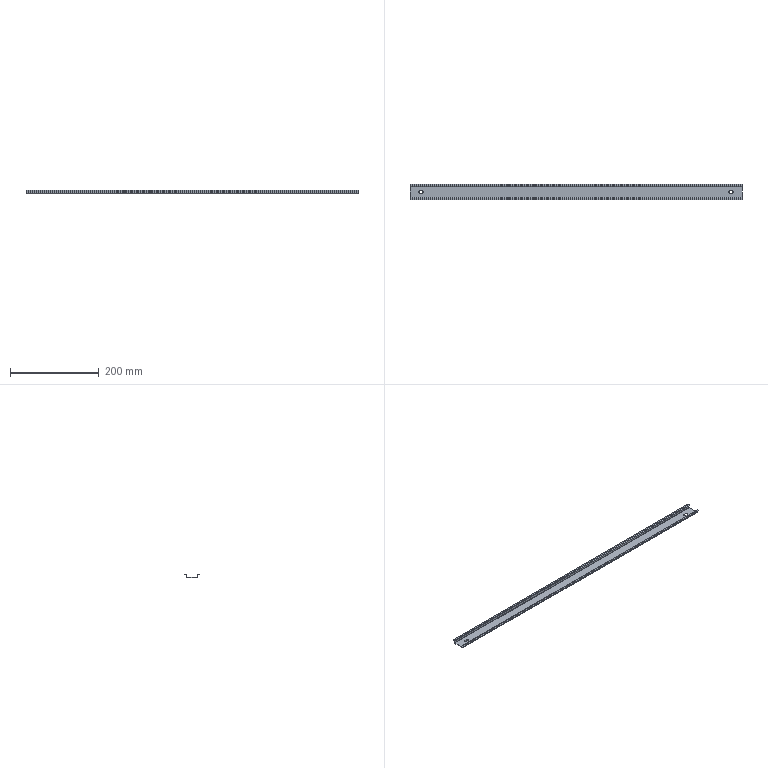Part | SolidWorks | features BaseBody 1 | 1 solid | 48 faces | box 750 x 35 x 7.5 mm | volume 34621 mm3 | plane 34 | cylinder 14 | commonest cylinder face diameters 5.5 x6 1 x4 3 x4
STEP:
#1=CARTESIAN_POINT('',(-352.,-2.75,0.));
#2=VERTEX_POINT('',#1);
#3=CARTESIAN_POINT('',(-348.,-2.75,0.));
#4=VERTEX_POINT('',#3);
#5=CARTESIAN_POINT('',(-352.,-2.75,0.));
#6=DIRECTION('',(1.,0.,0.));
#7=VECTOR('',#6,1000.);
#8=LINE('',#5,#7);
#9=EDGE_CURVE('',#2,#4,#8,.T.);
#10=ORIENTED_EDGE('',*,*,#9,.T.);
#11=CARTESIAN_POINT('',(-348.,-2.75,-1.));
#12=VERTEX_POINT('',#11);
#13=CARTESIAN_POINT('',(-348.,-2.75,-1.));
#14=DIRECTION('',(0.,0.,1.));
#15=VECTOR('',#14,1000.);
#16=LINE('',#13,#15);
#17=EDGE_CURVE('',#12,#4,#16,.T.);
#18=ORIENTED_EDGE('',*,*,#17,.F.);
#19=CARTESIAN_POINT('',(-352.,-2.75,-1.));
#20=VERTEX_POINT('',#19);
#21=CARTESIAN_POINT('',(-352.,-2.75,-1.));
#22=DIRECTION('',(1.,0.,0.));
#23=VECTOR('',#22,1000.);
#24=LINE('',#21,#23);
#25=EDGE_CURVE('',#20,#12,#24,.T.);
#26=ORIENTED_EDGE('',*,*,#25,.F.);
#27=CARTESIAN_POINT('',(-352.,-2.75,-1.));
#28=DIRECTION('',(0.,0.,1.));
#29=VECTOR('',#28,1000.);
#30=LINE('',#27,#29);
#31=EDGE_CURVE('',#20,#2,#30,.T.);
#32=ORIENTED_EDGE('',*,*,#31,.T.);
#33=EDGE_LOOP('',(#10,#18,#26,#32));
#34=FACE_OUTER_BOUND('',#33,.T.);
#35=CARTESIAN_POINT('',(-352.,-2.75,-1.));
#36=DIRECTION('',(0.,-1.,0.));
#37=DIRECTION('',(-1.,0.,0.));
#38=AXIS2_PLACEMENT_3D('',#35,#36,#37);
#39=PLANE('',#38);
#40=ADVANCED_FACE('',(#34),#39,.F.);
#41=CARTESIAN_POINT('',(-345.25,0.,-1.));
#42=VERTEX_POINT('',#41);
#43=CARTESIAN_POINT('',(-345.25,0.,0.));
#44=VERTEX_POINT('',#43);
#45=CARTESIAN_POINT('',(-345.25,0.,-1.));
#46=DIRECTION('',(0.,0.,1.));
#47=VECTOR('',#46,1000.);
#48=LINE('',#45,#47);
#49=EDGE_CURVE('',#42,#44,#48,.T.);
#50=ORIENTED_EDGE('',*,*,#49,.F.);
#51=CARTESIAN_POINT('',(-348.,0.,-1.));
#52=DIRECTION('',(0.,0.,1.));
#53=DIRECTION('',(1.,0.,0.));
#54=AXIS2_PLACEMENT_3D('',#51,#52,#53);
#55=CIRCLE('',#54,2.75);
#56=EDGE_CURVE('',#12,#42,#55,.T.);
#57=ORIENTED_EDGE('',*,*,#56,.F.);
#58=ORIENTED_EDGE('',*,*,#17,.T.);
#59=CARTESIAN_POINT('',(-348.,0.,0.));
#60=DIRECTION('',(0.,0.,1.));
#61=DIRECTION('',(1.,0.,0.));
#62=AXIS2_PLACEMENT_3D('',#59,#60,#61);
#63=CIRCLE('',#62,2.75);
#64=EDGE_CURVE('',#4,#44,#63,.T.);
#65=ORIENTED_EDGE('',*,*,#64,.T.);
#66=EDGE_LOOP('',(#50,#57,#58,#65));
#67=FACE_OUTER_BOUND('',#66,.T.);
#68=CARTESIAN_POINT('',(-348.,0.,-1.));
#69=DIRECTION('',(0.,0.,1.));
#70=DIRECTION('',(1.,0.,0.));
#71=AXIS2_PLACEMENT_3D('',#68,#69,#70);
#72=CYLINDRICAL_SURFACE('',#71,2.75);
#73=ADVANCED_FACE('',(#67),#72,.F.);
#74=CARTESIAN_POINT('',(-348.,2.75,0.));
#75=VERTEX_POINT('',#74);
#76=CARTESIAN_POINT('',(-352.,2.75,0.));
#77=VERTEX_POINT('',#76);
#78=CARTESIAN_POINT('',(-352.,2.75,0.));
#79=DIRECTION('',(-1.,0.,0.));
#80=VECTOR('',#79,1000.);
#81=LINE('',#78,#80);
#82=EDGE_CURVE('',#75,#77,#81,.T.);
#83=ORIENTED_EDGE('',*,*,#82,.T.);
#84=CARTESIAN_POINT('',(-352.,2.75,-1.));
#85=VERTEX_POINT('',#84);
#86=CARTESIAN_POINT('',(-352.,2.75,-1.));
#87=DIRECTION('',(0.,0.,1.));
#88=VECTOR('',#87,1000.);
#89=LINE('',#86,#88);
#90=EDGE_CURVE('',#85,#77,#89,.T.);
#91=ORIENTED_EDGE('',*,*,#90,.F.);
#92=CARTESIAN_POINT('',(-348.,2.75,-1.));
#93=VERTEX_POINT('',#92);
#94=CARTESIAN_POINT('',(-352.,2.75,-1.));
#95=DIRECTION('',(-1.,0.,0.));
#96=VECTOR('',#95,1000.);
#97=LINE('',#94,#96);
#98=EDGE_CURVE('',#93,#85,#97,.T.);
#99=ORIENTED_EDGE('',*,*,#98,.F.);
#100=CARTESIAN_POINT('',(-348.,2.75,-1.));
#101=DIRECTION('',(0.,0.,1.));
#102=VECTOR('',#101,1000.);
#103=LINE('',#100,#102);
#104=EDGE_CURVE('',#93,#75,#103,.T.);
#105=ORIENTED_EDGE('',*,*,#104,.T.);
#106=EDGE_LOOP('',(#83,#91,#99,#105));
#107=FACE_OUTER_BOUND('',#106,.T.);
#108=CARTESIAN_POINT('',(-352.,2.75,-1.));
#109=DIRECTION('',(0.,1.,0.));
#110=DIRECTION('',(1.,0.,0.));
#111=AXIS2_PLACEMENT_3D('',#108,#109,#110);
#112=PLANE('',#111);
#113=ADVANCED_FACE('',(#107),#112,.F.);
#114=CARTESIAN_POINT('',(-352.,0.,0.));
#115=DIRECTION('',(0.,0.,1.));
#116=DIRECTION('',(1.,0.,0.));
#117=AXIS2_PLACEMENT_3D('',#114,#115,#116);
#118=CIRCLE('',#117,2.75);
#119=EDGE_CURVE('',#77,#2,#118,.T.);
#120=ORIENTED_EDGE('',*,*,#119,.T.);
#121=ORIENTED_EDGE('',*,*,#31,.F.);
#122=CARTESIAN_POINT('',(-352.,0.,-1.));
#123=DIRECTION('',(0.,0.,1.));
#124=DIRECTION('',(1.,0.,0.));
#125=AXIS2_PLACEMENT_3D('',#122,#123,#124);
#126=CIRCLE('',#125,2.75);
#127=EDGE_CURVE('',#85,#20,#126,.T.);
#128=ORIENTED_EDGE('',*,*,#127,.F.);
#129=ORIENTED_EDGE('',*,*,#90,.T.);
#130=EDGE_LOOP('',(#120,#121,#128,#129));
#131=FACE_OUTER_BOUND('',#130,.T.);
#132=CARTESIAN_POINT('',(-352.,0.,-1.));
#133=DIRECTION('',(0.,0.,1.));
#134=DIRECTION('',(1.,0.,0.));
#135=AXIS2_PLACEMENT_3D('',#132,#133,#134);
#136=CYLINDRICAL_SURFACE('',#135,2.75);
#137=ADVANCED_FACE('',(#131),#136,.F.);
#138=CARTESIAN_POINT('',(352.,2.75,0.));
#139=VERTEX_POINT('',#138);
#140=CARTESIAN_POINT('',(348.,2.75,0.));
#141=VERTEX_POINT('',#140);
#142=CARTESIAN_POINT('',(352.,2.75,0.));
#143=DIRECTION('',(-1.,0.,0.));
#144=VECTOR('',#143,1000.);
#145=LINE('',#142,#144);
#146=EDGE_CURVE('',#139,#141,#145,.T.);
#147=ORIENTED_EDGE('',*,*,#146,.T.);
#148=CARTESIAN_POINT('',(348.,2.75,-1.));
#149=VERTEX_POINT('',#148);
#150=CARTESIAN_POINT('',(348.,2.75,-1.));
#151=DIRECTION('',(0.,0.,1.));
#152=VECTOR('',#151,1000.);
#153=LINE('',#150,#152);
#154=EDGE_CURVE('',#149,#141,#153,.T.);
#155=ORIENTED_EDGE('',*,*,#154,.F.);
#156=CARTESIAN_POINT('',(352.,2.75,-1.));
#157=VERTEX_POINT('',#156);
#158=CARTESIAN_POINT('',(352.,2.75,-1.));
#159=DIRECTION('',(-1.,0.,0.));
#160=VECTOR('',#159,1000.);
#161=LINE('',#158,#160);
#162=EDGE_CURVE('',#157,#149,#161,.T.);
#163=ORIENTED_EDGE('',*,*,#162,.F.);
#164=CARTESIAN_POINT('',(352.,2.75,-1.));
#165=DIRECTION('',(0.,0.,1.));
#166=VECTOR('',#165,1000.);
#167=LINE('',#164,#166);
#168=EDGE_CURVE('',#157,#139,#167,.T.);
#169=ORIENTED_EDGE('',*,*,#168,.T.);
#170=EDGE_LOOP('',(#147,#155,#163,#169));
#171=FACE_OUTER_BOUND('',#170,.T.);
#172=CARTESIAN_POINT('',(352.,2.75,-1.));
#173=DIRECTION('',(0.,1.,0.));
#174=DIRECTION('',(1.,0.,0.));
#175=AXIS2_PLACEMENT_3D('',#172,#173,#174);
#176=PLANE('',#175);
#177=ADVANCED_FACE('',(#171),#176,.F.);
#178=CARTESIAN_POINT('',(348.,-2.75,0.));
#179=VERTEX_POINT('',#178);
#180=CARTESIAN_POINT('',(348.,0.,0.));
#181=DIRECTION('',(0.,0.,1.));
#182=DIRECTION('',(-1.,0.,0.));
#183=AXIS2_PLACEMENT_3D('',#180,#181,#182);
#184=CIRCLE('',#183,2.75);
#185=EDGE_CURVE('',#141,#179,#184,.T.);
#186=ORIENTED_EDGE('',*,*,#185,.T.);
#187=CARTESIAN_POINT('',(348.,-2.75,-1.));
#188=VERTEX_POINT('',#187);
#189=CARTESIAN_POINT('',(348.,-2.75,-1.));
#190=DIRECTION('',(0.,0.,1.));
#191=VECTOR('',#190,1000.);
#192=LINE('',#189,#191);
#193=EDGE_CURVE('',#188,#179,#192,.T.);
#194=ORIENTED_EDGE('',*,*,#193,.F.);
#195=CARTESIAN_POINT('',(348.,0.,-1.));
#196=DIRECTION('',(0.,0.,1.));
#197=DIRECTION('',(-1.,0.,0.));
#198=AXIS2_PLACEMENT_3D('',#195,#196,#197);
#199=CIRCLE('',#198,2.75);
#200=EDGE_CURVE('',#149,#188,#199,.T.);
#201=ORIENTED_EDGE('',*,*,#200,.F.);
#202=ORIENTED_EDGE('',*,*,#154,.T.);
#203=EDGE_LOOP('',(#186,#194,#201,#202));
#204=FACE_OUTER_BOUND('',#203,.T.);
#205=CARTESIAN_POINT('',(348.,0.,-1.));
#206=DIRECTION('',(0.,0.,1.));
#207=DIRECTION('',(1.,0.,0.));
#208=AXIS2_PLACEMENT_3D('',#205,#206,#207);
#209=CYLINDRICAL_SURFACE('',#208,2.75);
#210=ADVANCED_FACE('',(#204),#209,.F.);
#211=CARTESIAN_POINT('',(352.,-2.75,0.));
#212=VERTEX_POINT('',#211);
#213=CARTESIAN_POINT('',(352.,-2.75,0.));
#214=DIRECTION('',(1.,0.,0.));
#215=VECTOR('',#214,1000.);
#216=LINE('',#213,#215);
#217=EDGE_CURVE('',#179,#212,#216,.T.);
#218=ORIENTED_EDGE('',*,*,#217,.T.);
#219=CARTESIAN_POINT('',(352.,-2.75,-1.));
#220=VERTEX_POINT('',#219);
#221=CARTESIAN_POINT('',(352.,-2.75,-1.));
#222=DIRECTION('',(0.,0.,1.));
#223=VECTOR('',#222,1000.);
#224=LINE('',#221,#223);
#225=EDGE_CURVE('',#220,#212,#224,.T.);
#226=ORIENTED_EDGE('',*,*,#225,.F.);
#227=CARTESIAN_POINT('',(352.,-2.75,-1.));
#228=DIRECTION('',(1.,0.,0.));
#229=VECTOR('',#228,1000.);
#230=LINE('',#227,#229);
#231=EDGE_CURVE('',#188,#220,#230,.T.);
#232=ORIENTED_EDGE('',*,*,#231,.F.);
#233=ORIENTED_EDGE('',*,*,#193,.T.);
#234=EDGE_LOOP('',(#218,#226,#232,#233));
#235=FACE_OUTER_BOUND('',#234,.T.);
#236=CARTESIAN_POINT('',(352.,-2.75,-1.));
#237=DIRECTION('',(0.,-1.,0.));
#238=DIRECTION('',(0.,0.,-1.));
#239=AXIS2_PLACEMENT_3D('',#236,#237,#238);
#240=PLANE('',#239);
#241=ADVANCED_FACE('',(#235),#240,.F.);
#242=CARTESIAN_POINT('',(354.75,0.,-1.));
#243=VERTEX_POINT('',#242);
#244=CARTESIAN_POINT('',(354.75,0.,0.));
#245=VERTEX_POINT('',#244);
#246=CARTESIAN_POINT('',(354.75,0.,-1.));
#247=DIRECTION('',(0.,0.,1.));
#248=VECTOR('',#247,1000.);
#249=LINE('',#246,#248);
#250=EDGE_CURVE('',#243,#245,#249,.T.);
#251=ORIENTED_EDGE('',*,*,#250,.F.);
#252=CARTESIAN_POINT('',(352.,0.,-1.));
#253=DIRECTION('',(0.,0.,1.));
#254=DIRECTION('',(-1.,0.,0.));
#255=AXIS2_PLACEMENT_3D('',#252,#253,#254);
#256=CIRCLE('',#255,2.75);
#257=EDGE_CURVE('',#220,#243,#256,.T.);
#258=ORIENTED_EDGE('',*,*,#257,.F.);
#259=ORIENTED_EDGE('',*,*,#225,.T.);
#260=CARTESIAN_POINT('',(352.,0.,0.));
#261=DIRECTION('',(0.,0.,1.));
#262=DIRECTION('',(-1.,0.,0.));
#263=AXIS2_PLACEMENT_3D('',#260,#261,#262);
#264=CIRCLE('',#263,2.75);
#265=EDGE_CURVE('',#212,#245,#264,.T.);
#266=ORIENTED_EDGE('',*,*,#265,.T.);
#267=EDGE_LOOP('',(#251,#258,#259,#266));
#268=FACE_OUTER_BOUND('',#267,.T.);
#269=CARTESIAN_POINT('',(352.,0.,-1.));
#270=DIRECTION('',(0.,0.,1.));
#271=DIRECTION('',(1.,0.,0.));
#272=AXIS2_PLACEMENT_3D('',#269,#270,#271);
#273=CYLINDRICAL_SURFACE('',#272,2.75);
#274=ADVANCED_FACE('',(#268),#273,.F.);
#275=CARTESIAN_POINT('',(-375.,-17.5,5.5));
#276=VERTEX_POINT('',#275);
#277=CARTESIAN_POINT('',(375.,-17.5,5.5));
#278=VERTEX_POINT('',#277);
#279=CARTESIAN_POINT('',(375.,-17.5,5.5));
#280=DIRECTION('',(1.,0.,0.));
#281=VECTOR('',#280,1000.);
#282=LINE('',#279,#281);
#283=EDGE_CURVE('',#276,#278,#282,.T.);
#284=ORIENTED_EDGE('',*,*,#283,.T.);
#285=CARTESIAN_POINT('',(375.,-17.5,6.5));
#286=VERTEX_POINT('',#285);
#287=CARTESIAN_POINT('',(375.,-17.5,6.5));
#288=DIRECTION('',(0.,0.,-1.));
#289=VECTOR('',#288,1000.);
#290=LINE('',#287,#289);
#291=EDGE_CURVE('',#286,#278,#290,.T.);
#292=ORIENTED_EDGE('',*,*,#291,.F.);
#293=CARTESIAN_POINT('',(-375.,-17.5,6.5));
#294=VERTEX_POINT('',#293);
#295=CARTESIAN_POINT('',(0.,-17.5,6.5));
#296=DIRECTION('',(1.,0.,0.));
#297=VECTOR('',#296,1000.);
#298=LINE('',#295,#297);
#299=EDGE_CURVE('',#294,#286,#298,.T.);
#300=ORIENTED_EDGE('',*,*,#299,.F.);
#301=CARTESIAN_POINT('',(-375.,-17.5,6.5));
#302=DIRECTION('',(0.,0.,-1.));
#303=VECTOR('',#302,1000.);
#304=LINE('',#301,#303);
#305=EDGE_CURVE('',#294,#276,#304,.T.);
#306=ORIENTED_EDGE('',*,*,#305,.T.);
#307=EDGE_LOOP('',(#284,#292,#300,#306));
#308=FACE_OUTER_BOUND('',#307,.T.);
#309=CARTESIAN_POINT('',(375.,-17.5,6.5));
#310=DIRECTION('',(0.,1.,0.));
#311=DIRECTION('',(0.,0.,-1.));
#312=AXIS2_PLACEMENT_3D('',#309,#310,#311);
#313=PLANE('',#312);
#314=ADVANCED_FACE('',(#308),#313,.F.);
#315=CARTESIAN_POINT('',(-375.,-14.,5.5));
#316=VERTEX_POINT('',#315);
#317=CARTESIAN_POINT('',(-375.,-17.5,5.5));
#318=DIRECTION('',(0.,-1.,0.));
#319=VECTOR('',#318,1000.);
#320=LINE('',#317,#319);
#321=EDGE_CURVE('',#316,#276,#320,.T.);
#322=ORIENTED_EDGE('',*,*,#321,.F.);
#323=CARTESIAN_POINT('',(375.,-14.,5.5));
#324=VERTEX_POINT('',#323);
#325=CARTESIAN_POINT('',(375.,-14.,5.5));
#326=DIRECTION('',(-1.,0.,0.));
#327=VECTOR('',#326,1000.);
#328=LINE('',#325,#327);
#329=EDGE_CURVE('',#324,#316,#328,.T.);
#330=ORIENTED_EDGE('',*,*,#329,.F.);
#331=CARTESIAN_POINT('',(375.,-13.5,5.5));
#332=DIRECTION('',(0.,1.,0.));
#333=VECTOR('',#332,1000.);
#334=LINE('',#331,#333);
#335=EDGE_CURVE('',#278,#324,#334,.T.);
#336=ORIENTED_EDGE('',*,*,#335,.F.);
#337=ORIENTED_EDGE('',*,*,#283,.F.);
#338=EDGE_LOOP('',(#322,#330,#336,#337));
#339=FACE_OUTER_BOUND('',#338,.T.);
#340=CARTESIAN_POINT('',(0.,0.,5.5));
#341=DIRECTION('',(0.,0.,-1.));
#342=DIRECTION('',(-1.,0.,0.));
#343=AXIS2_PLACEMENT_3D('',#340,#341,#342);
#344=PLANE('',#343);
#345=ADVANCED_FACE('',(#339),#344,.T.);
#346=CARTESIAN_POINT('',(-375.,-14.,6.5));
#347=VERTEX_POINT('',#346);
#348=CARTESIAN_POINT('',(375.,-14.,6.5));
#349=VERTEX_POINT('',#348);
#350=CARTESIAN_POINT('',(375.,-14.,6.5));
#351=DIRECTION('',(1.,0.,0.));
#352=VECTOR('',#351,1000.);
#353=LINE('',#350,#352);
#354=EDGE_CURVE('',#347,#349,#353,.T.);
#355=ORIENTED_EDGE('',*,*,#354,.F.);
#356=CARTESIAN_POINT('',(-375.,0.,6.5));
#357=DIRECTION('',(0.,-1.,0.));
#358=VECTOR('',#357,1000.);
#359=LINE('',#356,#358);
#360=EDGE_CURVE('',#347,#294,#359,.T.);
#361=ORIENTED_EDGE('',*,*,#360,.T.);
#362=ORIENTED_EDGE('',*,*,#299,.T.);
#363=CARTESIAN_POINT('',(375.,0.,6.5));
#364=DIRECTION('',(0.,1.,0.));
#365=VECTOR('',#364,1000.);
#366=LINE('',#363,#365);
#367=EDGE_CURVE('',#286,#349,#366,.T.);
#368=ORIENTED_EDGE('',*,*,#367,.T.);
#369=EDGE_LOOP('',(#355,#361,#362,#368));
#370=FACE_OUTER_BOUND('',#369,.T.);
#371=CARTESIAN_POINT('',(0.,0.,6.5));
#372=DIRECTION('',(0.,0.,-1.));
#373=DIRECTION('',(-1.,0.,0.));
#374=AXIS2_PLACEMENT_3D('',#371,#372,#373);
#375=PLANE('',#374);
#376=ADVANCED_FACE('',(#370),#375,.F.);
#377=CARTESIAN_POINT('',(-375.,-14.,5.5));
#378=DIRECTION('',(0.,0.,1.));
#379=VECTOR('',#378,1000.);
#380=LINE('',#377,#379);
#381=EDGE_CURVE('',#316,#347,#380,.T.);
#382=ORIENTED_EDGE('',*,*,#381,.F.);
#383=ORIENTED_EDGE('',*,*,#321,.T.);
#384=ORIENTED_EDGE('',*,*,#305,.F.);
#385=ORIENTED_EDGE('',*,*,#360,.F.);
#386=EDGE_LOOP('',(#382,#383,#384,#385));
#387=FACE_OUTER_BOUND('',#386,.T.);
#388=CARTESIAN_POINT('',(-375.,-17.5,6.5));
#389=DIRECTION('',(1.,0.,0.));
#390=DIRECTION('',(0.,0.,-1.));
#391=AXIS2_PLACEMENT_3D('',#388,#389,#390);
#392=PLANE('',#391);
#393=ADVANCED_FACE('',(#387),#392,.F.);
#394=CARTESIAN_POINT('',(375.,-14.,6.5));
#395=DIRECTION('',(0.,0.,1.));
#396=VECTOR('',#395,1000.);
#397=LINE('',#394,#396);
#398=EDGE_CURVE('',#324,#349,#397,.T.);
#399=ORIENTED_EDGE('',*,*,#398,.T.);
#400=ORIENTED_EDGE('',*,*,#367,.F.);
#401=ORIENTED_EDGE('',*,*,#291,.T.);
#402=ORIENTED_EDGE('',*,*,#335,.T.);
#403=EDGE_LOOP('',(#399,#400,#401,#402));
#404=FACE_OUTER_BOUND('',#403,.T.);
#405=CARTESIAN_POINT('',(375.,-13.5,6.5));
#406=DIRECTION('',(-1.,0.,0.));
#407=DIRECTION('',(0.,1.,0.));
#408=AXIS2_PLACEMENT_3D('',#405,#406,#407);
#409=PLANE('',#408);
#410=ADVANCED_FACE('',(#404),#409,.F.);
#411=CARTESIAN_POINT('',(-375.,-13.5,5.));
#412=VERTEX_POINT('',#411);
#413=CARTESIAN_POINT('',(375.,-13.5,5.));
#414=VERTEX_POINT('',#413);
#415=CARTESIAN_POINT('',(-375.,-13.5,5.));
#416=DIRECTION('',(1.,0.,0.));
#417=VECTOR('',#416,1000.);
#418=LINE('',#415,#417);
#419=EDGE_CURVE('',#412,#414,#418,.T.);
#420=ORIENTED_EDGE('',*,*,#419,.T.);
#421=CARTESIAN_POINT('',(375.,-14.,5.));
#422=DIRECTION('',(1.,0.,0.));
#423=DIRECTION('',(0.,0.,1.));
#424=AXIS2_PLACEMENT_3D('',#421,#422,#423);
#425=CIRCLE('',#424,0.5);
#426=EDGE_CURVE('',#414,#324,#425,.T.);
#427=ORIENTED_EDGE('',*,*,#426,.T.);
#428=ORIENTED_EDGE('',*,*,#329,.T.);
#429=CARTESIAN_POINT('',(-375.,-14.,5.));
#430=DIRECTION('',(-1.,0.,0.));
#431=DIRECTION('',(0.,0.,1.));
#432=AXIS2_PLACEMENT_3D('',#429,#430,#431);
#433=CIRCLE('',#432,0.5);
#434=EDGE_CURVE('',#316,#412,#433,.T.);
#435=ORIENTED_EDGE('',*,*,#434,.T.);
#436=EDGE_LOOP('',(#420,#427,#428,#435));
#437=FACE_OUTER_BOUND('',#436,.T.);
#438=CARTESIAN_POINT('',(-375.,-14.,5.));
#439=DIRECTION('',(-1.,0.,0.));
#440=DIRECTION('',(0.,0.,1.));
#441=AXIS2_PLACEMENT_3D('',#438,#439,#440);
#442=CYLINDRICAL_SURFACE('',#441,0.5);
#443=ADVANCED_FACE('',(#437),#442,.F.);
#444=CARTESIAN_POINT('',(-375.,-12.5,5.));
#445=VERTEX_POINT('',#444);
#446=CARTESIAN_POINT('',(375.,-12.5,5.));
#447=VERTEX_POINT('',#446);
#448=CARTESIAN_POINT('',(-375.,-12.5,5.));
#449=DIRECTION('',(1.,0.,0.));
#450=VECTOR('',#449,1000.);
#451=LINE('',#448,#450);
#452=EDGE_CURVE('',#445,#447,#451,.T.);
#453=ORIENTED_EDGE('',*,*,#452,.F.);
#454=CARTESIAN_POINT('',(-375.,-14.,5.));
#455=DIRECTION('',(-1.,0.,0.));
#456=DIRECTION('',(0.,0.,1.));
#457=AXIS2_PLACEMENT_3D('',#454,#455,#456);
#458=CIRCLE('',#457,1.5);
#459=EDGE_CURVE('',#347,#445,#458,.T.);
#460=ORIENTED_EDGE('',*,*,#459,.F.);
#461=ORIENTED_EDGE('',*,*,#354,.T.);
#462=CARTESIAN_POINT('',(375.,-14.,5.));
#463=DIRECTION('',(1.,0.,0.));
#464=DIRECTION('',(0.,0.,1.));
#465=AXIS2_PLACEMENT_3D('',#462,#463,#464);
#466=CIRCLE('',#465,1.5);
#467=EDGE_CURVE('',#447,#349,#466,.T.);
#468=ORIENTED_EDGE('',*,*,#467,.F.);
#469=EDGE_LOOP('',(#453,#460,#461,#468));
#470=FACE_OUTER_BOUND('',#469,.T.);
#471=CARTESIAN_POINT('',(-375.,-14.,5.));
#472=DIRECTION('',(-1.,0.,0.));
#473=DIRECTION('',(0.,0.,1.));
#474=AXIS2_PLACEMENT_3D('',#471,#472,#473);
#475=CYLINDRICAL_SURFACE('',#474,1.5);
#476=ADVANCED_FACE('',(#470),#475,.T.);
#477=ORIENTED_EDGE('',*,*,#434,.F.);
#478=ORIENTED_EDGE('',*,*,#381,.T.);
#479=ORIENTED_EDGE('',*,*,#459,.T.);
#480=CARTESIAN_POINT('',(-375.,-13.5,5.));
#481=DIRECTION('',(0.,1.,0.));
#482=VECTOR('',#481,1000.);
#483=LINE('',#480,#482);
#484=EDGE_CURVE('',#412,#445,#483,.T.);
#485=ORIENTED_EDGE('',*,*,#484,.F.);
#486=EDGE_LOOP('',(#477,#478,#479,#485));
#487=FACE_OUTER_BOUND('',#486,.T.);
#488=CARTESIAN_POINT('',(-375.,-14.,5.));
#489=DIRECTION('',(1.,0.,0.));
#490=DIRECTION('',(0.,1.,0.));
#491=AXIS2_PLACEMENT_3D('',#488,#489,#490);
#492=PLANE('',#491);
#493=ADVANCED_FACE('',(#487),#492,.F.);
#494=ORIENTED_EDGE('',*,*,#398,.F.);
#495=ORIENTED_EDGE('',*,*,#426,.F.);
#496=CARTESIAN_POINT('',(375.,-13.5,5.));
#497=DIRECTION('',(0.,1.,0.));
#498=VECTOR('',#497,1000.);
#499=LINE('',#496,#498);
#500=EDGE_CURVE('',#414,#447,#499,.T.);
#501=ORIENTED_EDGE('',*,*,#500,.T.);
#502=ORIENTED_EDGE('',*,*,#467,.T.);
#503=EDGE_LOOP('',(#494,#495,#501,#502));
#504=FACE_OUTER_BOUND('',#503,.T.);
#505=CARTESIAN_POINT('',(375.,-14.,5.));
#506=DIRECTION('',(1.,0.,0.));
#507=DIRECTION('',(0.,1.,0.));
#508=AXIS2_PLACEMENT_3D('',#505,#506,#507);
#509=PLANE('',#508);
#510=ADVANCED_FACE('',(#504),#509,.T.);
#511=CARTESIAN_POINT('',(375.,17.5,5.5));
#512=VERTEX_POINT('',#511);
#513=CARTESIAN_POINT('',(-375.,17.5,5.5));
#514=VERTEX_POINT('',#513);
#515=CARTESIAN_POINT('',(-375.,17.5,5.5));
#516=DIRECTION('',(-1.,0.,0.));
#517=VECTOR('',#516,1000.);
#518=LINE('',#515,#517);
#519=EDGE_CURVE('',#512,#514,#518,.T.);
#520=ORIENTED_EDGE('',*,*,#519,.T.);
#521=CARTESIAN_POINT('',(-375.,17.5,6.5));
#522=VERTEX_POINT('',#521);
#523=CARTESIAN_POINT('',(-375.,17.5,6.5));
#524=DIRECTION('',(0.,0.,-1.));
#525=VECTOR('',#524,1000.);
#526=LINE('',#523,#525);
#527=EDGE_CURVE('',#522,#514,#526,.T.);
#528=ORIENTED_EDGE('',*,*,#527,.F.);
#529=CARTESIAN_POINT('',(375.,17.5,6.5));
#530=VERTEX_POINT('',#529);
#531=CARTESIAN_POINT('',(0.,17.5,6.5));
#532=DIRECTION('',(-1.,0.,0.));
#533=VECTOR('',#532,1000.);
#534=LINE('',#531,#533);
#535=EDGE_CURVE('',#530,#522,#534,.T.);
#536=ORIENTED_EDGE('',*,*,#535,.F.);
#537=CARTESIAN_POINT('',(375.,17.5,6.5));
#538=DIRECTION('',(0.,0.,-1.));
#539=VECTOR('',#538,1000.);
#540=LINE('',#537,#539);
#541=EDGE_CURVE('',#530,#512,#540,.T.);
#542=ORIENTED_EDGE('',*,*,#541,.T.);
#543=EDGE_LOOP('',(#520,#528,#536,#542));
#544=FACE_OUTER_BOUND('',#543,.T.);
#545=CARTESIAN_POINT('',(-375.,17.5,6.5));
#546=DIRECTION('',(0.,-1.,0.));
#547=DIRECTION('',(0.,0.,-1.));
#548=AXIS2_PLACEMENT_3D('',#545,#546,#547);
#549=PLANE('',#548);
#550=ADVANCED_FACE('',(#544),#549,.F.);
#551=CARTESIAN_POINT('',(375.,14.,5.5));
#552=VERTEX_POINT('',#551);
#553=CARTESIAN_POINT('',(375.,17.5,5.5));
#554=DIRECTION('',(0.,1.,0.));
#555=VECTOR('',#554,1000.);
#556=LINE('',#553,#555);
#557=EDGE_CURVE('',#552,#512,#556,.T.);
#558=ORIENTED_EDGE('',*,*,#557,.F.);
#559=CARTESIAN_POINT('',(-375.,14.,5.5));
#560=VERTEX_POINT('',#559);
#561=CARTESIAN_POINT('',(-375.,14.,5.5));
#562=DIRECTION('',(1.,0.,0.));
#563=VECTOR('',#562,1000.);
#564=LINE('',#561,#563);
#565=EDGE_CURVE('',#560,#552,#564,.T.);
#566=ORIENTED_EDGE('',*,*,#565,.F.);
#567=CARTESIAN_POINT('',(-375.,13.5,5.5));
#568=DIRECTION('',(0.,-1.,0.));
#569=VECTOR('',#568,1000.);
#570=LINE('',#567,#569);
#571=EDGE_CURVE('',#514,#560,#570,.T.);
#572=ORIENTED_EDGE('',*,*,#571,.F.);
#573=ORIENTED_EDGE('',*,*,#519,.F.);
#574=EDGE_LOOP('',(#558,#566,#572,#573));
#575=FACE_OUTER_BOUND('',#574,.T.);
#576=CARTESIAN_POINT('',(0.,0.,5.5));
#577=DIRECTION('',(0.,0.,-1.));
#578=DIRECTION('',(0.,-1.,0.));
#579=AXIS2_PLACEMENT_3D('',#576,#577,#578);
#580=PLANE('',#579);
#581=ADVANCED_FACE('',(#575),#580,.T.);
#582=CARTESIAN_POINT('',(375.,14.,6.5));
#583=VERTEX_POINT('',#582);
#584=CARTESIAN_POINT('',(-375.,14.,6.5));
#585=VERTEX_POINT('',#584);
#586=CARTESIAN_POINT('',(-375.,14.,6.5));
#587=DIRECTION('',(-1.,0.,0.));
#588=VECTOR('',#587,1000.);
#589=LINE('',#586,#588);
#590=EDGE_CURVE('',#583,#585,#589,.T.);
#591=ORIENTED_EDGE('',*,*,#590,.F.);
#592=CARTESIAN_POINT('',(375.,0.,6.5));
#593=DIRECTION('',(0.,1.,0.));
#594=VECTOR('',#593,1000.);
#595=LINE('',#592,#594);
#596=EDGE_CURVE('',#583,#530,#595,.T.);
#597=ORIENTED_EDGE('',*,*,#596,.T.);
#598=ORIENTED_EDGE('',*,*,#535,.T.);
#599=CARTESIAN_POINT('',(-375.,0.,6.5));
#600=DIRECTION('',(0.,-1.,0.));
#601=VECTOR('',#600,1000.);
#602=LINE('',#599,#601);
#603=EDGE_CURVE('',#522,#585,#602,.T.);
#604=ORIENTED_EDGE('',*,*,#603,.T.);
#605=EDGE_LOOP('',(#591,#597,#598,#604));
#606=FACE_OUTER_BOUND('',#605,.T.);
#607=CARTESIAN_POINT('',(0.,0.,6.5));
#608=DIRECTION('',(0.,0.,-1.));
#609=DIRECTION('',(0.,-1.,0.));
#610=AXIS2_PLACEMENT_3D('',#607,#608,#609);
#611=PLANE('',#610);
#612=ADVANCED_FACE('',(#606),#611,.F.);
#613=CARTESIAN_POINT('',(375.,14.,5.5));
#614=DIRECTION('',(0.,0.,1.));
#615=VECTOR('',#614,1000.);
#616=LINE('',#613,#615);
#617=EDGE_CURVE('',#552,#583,#616,.T.);
#618=ORIENTED_EDGE('',*,*,#617,.F.);
#619=ORIENTED_EDGE('',*,*,#557,.T.);
#620=ORIENTED_EDGE('',*,*,#541,.F.);
#621=ORIENTED_EDGE('',*,*,#596,.F.);
#622=EDGE_LOOP('',(#618,#619,#620,#621));
#623=FACE_OUTER_BOUND('',#622,.T.);
#624=CARTESIAN_POINT('',(375.,17.5,6.5));
#625=DIRECTION('',(-1.,0.,0.));
#626=DIRECTION('',(0.,0.,1.));
#627=AXIS2_PLACEMENT_3D('',#624,#625,#626);
#628=PLANE('',#627);
#629=ADVANCED_FACE('',(#623),#628,.F.);
#630=CARTESIAN_POINT('',(-375.,14.,6.5));
#631=DIRECTION('',(0.,0.,1.));
#632=VECTOR('',#631,1000.);
#633=LINE('',#630,#632);
#634=EDGE_CURVE('',#560,#585,#633,.T.);
#635=ORIENTED_EDGE('',*,*,#634,.T.);
#636=ORIENTED_EDGE('',*,*,#603,.F.);
#637=ORIENTED_EDGE('',*,*,#527,.T.);
#638=ORIENTED_EDGE('',*,*,#571,.T.);
#639=EDGE_LOOP('',(#635,#636,#637,#638));
#640=FACE_OUTER_BOUND('',#639,.T.);
#641=CARTESIAN_POINT('',(-375.,13.5,6.5));
#642=DIRECTION('',(1.,0.,0.));
#643=DIRECTION('',(0.,1.,0.));
#644=AXIS2_PLACEMENT_3D('',#641,#642,#643);
#645=PLANE('',#644);
#646=ADVANCED_FACE('',(#640),#645,.F.);
#647=CARTESIAN_POINT('',(375.,13.5,5.));
#648=VERTEX_POINT('',#647);
#649=CARTESIAN_POINT('',(-375.,13.5,5.));
#650=VERTEX_POINT('',#649);
#651=CARTESIAN_POINT('',(375.,13.5,5.));
#652=DIRECTION('',(-1.,0.,0.));
#653=VECTOR('',#652,1000.);
#654=LINE('',#651,#653);
#655=EDGE_CURVE('',#648,#650,#654,.T.);
#656=ORIENTED_EDGE('',*,*,#655,.T.);
#657=CARTESIAN_POINT('',(-375.,14.,5.));
#658=DIRECTION('',(-1.,0.,0.));
#659=DIRECTION('',(0.,0.,-1.));
#660=AXIS2_PLACEMENT_3D('',#657,#658,#659);
#661=CIRCLE('',#660,0.5);
#662=EDGE_CURVE('',#650,#560,#661,.T.);
#663=ORIENTED_EDGE('',*,*,#662,.T.);
#664=ORIENTED_EDGE('',*,*,#565,.T.);
#665=CARTESIAN_POINT('',(375.,14.,5.));
#666=DIRECTION('',(1.,0.,0.));
#667=DIRECTION('',(0.,0.,-1.));
#668=AXIS2_PLACEMENT_3D('',#665,#666,#667);
#669=CIRCLE('',#668,0.5);
#670=EDGE_CURVE('',#552,#648,#669,.T.);
#671=ORIENTED_EDGE('',*,*,#670,.T.);
#672=EDGE_LOOP('',(#656,#663,#664,#671));
#673=FACE_OUTER_BOUND('',#672,.T.);
#674=CARTESIAN_POINT('',(375.,14.,5.));
#675=DIRECTION('',(1.,0.,0.));
#676=DIRECTION('',(0.,0.,1.));
#677=AXIS2_PLACEMENT_3D('',#674,#675,#676);
#678=CYLINDRICAL_SURFACE('',#677,0.5);
#679=ADVANCED_FACE('',(#673),#678,.F.);
#680=CARTESIAN_POINT('',(375.,12.5,5.));
#681=VERTEX_POINT('',#680);
#682=CARTESIAN_POINT('',(-375.,12.5,5.));
#683=VERTEX_POINT('',#682);
#684=CARTESIAN_POINT('',(375.,12.5,5.));
#685=DIRECTION('',(-1.,0.,0.));
#686=VECTOR('',#685,1000.);
#687=LINE('',#684,#686);
#688=EDGE_CURVE('',#681,#683,#687,.T.);
#689=ORIENTED_EDGE('',*,*,#688,.F.);
#690=CARTESIAN_POINT('',(375.,14.,5.));
#691=DIRECTION('',(1.,0.,0.));
#692=DIRECTION('',(0.,0.,-1.));
#693=AXIS2_PLACEMENT_3D('',#690,#691,#692);
#694=CIRCLE('',#693,1.5);
#695=EDGE_CURVE('',#583,#681,#694,.T.);
#696=ORIENTED_EDGE('',*,*,#695,.F.);
#697=ORIENTED_EDGE('',*,*,#590,.T.);
#698=CARTESIAN_POINT('',(-375.,14.,5.));
#699=DIRECTION('',(-1.,0.,0.));
#700=DIRECTION('',(0.,0.,-1.));
#701=AXIS2_PLACEMENT_3D('',#698,#699,#700);
#702=CIRCLE('',#701,1.5);
#703=EDGE_CURVE('',#683,#585,#702,.T.);
#704=ORIENTED_EDGE('',*,*,#703,.F.);
#705=EDGE_LOOP('',(#689,#696,#697,#704));
#706=FACE_OUTER_BOUND('',#705,.T.);
#707=CARTESIAN_POINT('',(375.,14.,5.));
#708=DIRECTION('',(1.,0.,0.));
#709=DIRECTION('',(0.,0.,1.));
#710=AXIS2_PLACEMENT_3D('',#707,#708,#709);
#711=CYLINDRICAL_SURFACE('',#710,1.5);
#712=ADVANCED_FACE('',(#706),#711,.T.);
#713=ORIENTED_EDGE('',*,*,#670,.F.);
#714=ORIENTED_EDGE('',*,*,#617,.T.);
#715=ORIENTED_EDGE('',*,*,#695,.T.);
#716=CARTESIAN_POINT('',(375.,13.5,5.));
#717=DIRECTION('',(0.,-1.,0.));
#718=VECTOR('',#717,1000.);
#719=LINE('',#716,#718);
#720=EDGE_CURVE('',#648,#681,#719,.T.);
#721=ORIENTED_EDGE('',*,*,#720,.F.);
#722=EDGE_LOOP('',(#713,#714,#715,#721));
#723=FACE_OUTER_BOUND('',#722,.T.);
#724=CARTESIAN_POINT('',(375.,14.,5.));
#725=DIRECTION('',(-1.,0.,0.));
#726=DIRECTION('',(0.,0.,1.));
#727=AXIS2_PLACEMENT_3D('',#724,#725,#726);
#728=PLANE('',#727);
#729=ADVANCED_FACE('',(#723),#728,.F.);
#730=ORIENTED_EDGE('',*,*,#634,.F.);
#731=ORIENTED_EDGE('',*,*,#662,.F.);
#732=CARTESIAN_POINT('',(-375.,13.5,5.));
#733=DIRECTION('',(0.,-1.,0.));
#734=VECTOR('',#733,1000.);
#735=LINE('',#732,#734);
#736=EDGE_CURVE('',#650,#683,#735,.T.);
#737=ORIENTED_EDGE('',*,*,#736,.T.);
#738=ORIENTED_EDGE('',*,*,#703,.T.);
#739=EDGE_LOOP('',(#730,#731,#737,#738));
#740=FACE_OUTER_BOUND('',#739,.T.);
#741=CARTESIAN_POINT('',(-375.,14.,5.));
#742=DIRECTION('',(-1.,0.,0.));
#743=DIRECTION('',(0.,0.,1.));
#744=AXIS2_PLACEMENT_3D('',#741,#742,#743);
#745=PLANE('',#744);
#746=ADVANCED_FACE('',(#740),#745,.T.);
#747=CARTESIAN_POINT('',(375.,-12.,0.));
#748=VERTEX_POINT('',#747);
#749=CARTESIAN_POINT('',(-375.,-12.,0.));
#750=VERTEX_POINT('',#749);
#751=CARTESIAN_POINT('',(375.,-12.,0.));
#752=DIRECTION('',(-1.,0.,0.));
#753=VECTOR('',#752,1000.);
#754=LINE('',#751,#753);
#755=EDGE_CURVE('',#748,#750,#754,.T.);
#756=ORIENTED_EDGE('',*,*,#755,.T.);
#757=CARTESIAN_POINT('',(-375.,-12.5,0.5));
#758=VERTEX_POINT('',#757);
#759=CARTESIAN_POINT('',(-375.,-12.,0.5));
#760=DIRECTION('',(-1.,0.,0.));
#761=DIRECTION('',(0.,0.,-1.));
#762=AXIS2_PLACEMENT_3D('',#759,#760,#761);
#763=CIRCLE('',#762,0.5);
#764=EDGE_CURVE('',#750,#758,#763,.T.);
#765=ORIENTED_EDGE('',*,*,#764,.T.);
#766=CARTESIAN_POINT('',(375.,-12.5,0.5));
#767=VERTEX_POINT('',#766);
#768=CARTESIAN_POINT('',(-375.,-12.5,0.5));
#769=DIRECTION('',(1.,0.,0.));
#770=VECTOR('',#769,1000.);
#771=LINE('',#768,#770);
#772=EDGE_CURVE('',#758,#767,#771,.T.);
#773=ORIENTED_EDGE('',*,*,#772,.T.);
#774=CARTESIAN_POINT('',(375.,-12.,0.5));
#775=DIRECTION('',(1.,0.,0.));
#776=DIRECTION('',(0.,0.,-1.));
#777=AXIS2_PLACEMENT_3D('',#774,#775,#776);
#778=CIRCLE('',#777,0.5);
#779=EDGE_CURVE('',#767,#748,#778,.T.);
#780=ORIENTED_EDGE('',*,*,#779,.T.);
#781=EDGE_LOOP('',(#756,#765,#773,#780));
#782=FACE_OUTER_BOUND('',#781,.T.);
#783=CARTESIAN_POINT('',(375.,-12.,0.5));
#784=DIRECTION('',(1.,0.,0.));
#785=DIRECTION('',(0.,-1.,0.));
#786=AXIS2_PLACEMENT_3D('',#783,#784,#785);
#787=CYLINDRICAL_SURFACE('',#786,0.5);
#788=ADVANCED_FACE('',(#782),#787,.F.);
#789=CARTESIAN_POINT('',(375.,-12.,-1.));
#790=VERTEX_POINT('',#789);
#791=CARTESIAN_POINT('',(-375.,-12.,-1.));
#792=VERTEX_POINT('',#791);
#793=CARTESIAN_POINT('',(375.,-12.,-1.));
#794=DIRECTION('',(-1.,0.,0.));
#795=VECTOR('',#794,1000.);
#796=LINE('',#793,#795);
#797=EDGE_CURVE('',#790,#792,#796,.T.);
#798=ORIENTED_EDGE('',*,*,#797,.F.);
#799=CARTESIAN_POINT('',(375.,-13.5,0.5));
#800=VERTEX_POINT('',#799);
#801=CARTESIAN_POINT('',(375.,-12.,0.5));
#802=DIRECTION('',(1.,0.,0.));
#803=DIRECTION('',(0.,0.,-1.));
#804=AXIS2_PLACEMENT_3D('',#801,#802,#803);
#805=CIRCLE('',#804,1.5);
#806=EDGE_CURVE('',#800,#790,#805,.T.);
#807=ORIENTED_EDGE('',*,*,#806,.F.);
#808=CARTESIAN_POINT('',(-375.,-13.5,0.5));
#809=VERTEX_POINT('',#808);
#810=CARTESIAN_POINT('',(-375.,-13.5,0.5));
#811=DIRECTION('',(-1.,0.,0.));
#812=VECTOR('',#811,1000.);
#813=LINE('',#810,#812);
#814=EDGE_CURVE('',#800,#809,#813,.T.);
#815=ORIENTED_EDGE('',*,*,#814,.T.);
#816=CARTESIAN_POINT('',(-375.,-12.,0.5));
#817=DIRECTION('',(-1.,0.,0.));
#818=DIRECTION('',(0.,0.,-1.));
#819=AXIS2_PLACEMENT_3D('',#816,#817,#818);
#820=CIRCLE('',#819,1.5);
#821=EDGE_CURVE('',#792,#809,#820,.T.);
#822=ORIENTED_EDGE('',*,*,#821,.F.);
#823=EDGE_LOOP('',(#798,#807,#815,#822));
#824=FACE_OUTER_BOUND('',#823,.T.);
#825=CARTESIAN_POINT('',(375.,-12.,0.5));
#826=DIRECTION('',(1.,0.,0.));
#827=DIRECTION('',(0.,-1.,0.));
#828=AXIS2_PLACEMENT_3D('',#825,#826,#827);
#829=CYLINDRICAL_SURFACE('',#828,1.5);
#830=ADVANCED_FACE('',(#824),#829,.T.);
#831=ORIENTED_EDGE('',*,*,#779,.F.);
#832=CARTESIAN_POINT('',(375.,-12.5,0.5));
#833=DIRECTION('',(0.,-1.,0.));
#834=VECTOR('',#833,1000.);
#835=LINE('',#832,#834);
#836=EDGE_CURVE('',#767,#800,#835,.T.);
#837=ORIENTED_EDGE('',*,*,#836,.T.);
#838=ORIENTED_EDGE('',*,*,#806,.T.);
#839=CARTESIAN_POINT('',(375.,-12.,0.));
#840=DIRECTION('',(0.,0.,-1.));
#841=VECTOR('',#840,1000.);
#842=LINE('',#839,#841);
#843=EDGE_CURVE('',#748,#790,#842,.T.);
#844=ORIENTED_EDGE('',*,*,#843,.F.);
#845=EDGE_LOOP('',(#831,#837,#838,#844));
#846=FACE_OUTER_BOUND('',#845,.T.);
#847=CARTESIAN_POINT('',(375.,-12.,0.5));
#848=DIRECTION('',(-1.,0.,0.));
#849=DIRECTION('',(0.,0.,1.));
#850=AXIS2_PLACEMENT_3D('',#847,#848,#849);
#851=PLANE('',#850);
#852=ADVANCED_FACE('',(#846),#851,.F.);
#853=CARTESIAN_POINT('',(-375.,-13.5,0.5));
#854=DIRECTION('',(0.,-1.,0.));
#855=VECTOR('',#854,1000.);
#856=LINE('',#853,#855);
#857=EDGE_CURVE('',#758,#809,#856,.T.);
#858=ORIENTED_EDGE('',*,*,#857,.F.);
#859=ORIENTED_EDGE('',*,*,#764,.F.);
#860=CARTESIAN_POINT('',(-375.,-12.,0.));
#861=DIRECTION('',(0.,0.,-1.));
#862=VECTOR('',#861,1000.);
#863=LINE('',#860,#862);
#864=EDGE_CURVE('',#750,#792,#863,.T.);
#865=ORIENTED_EDGE('',*,*,#864,.T.);
#866=ORIENTED_EDGE('',*,*,#821,.T.);
#867=EDGE_LOOP('',(#858,#859,#865,#866));
#868=FACE_OUTER_BOUND('',#867,.T.);
#869=CARTESIAN_POINT('',(-375.,-12.,0.5));
#870=DIRECTION('',(-1.,0.,0.));
#871=DIRECTION('',(0.,0.,1.));
#872=AXIS2_PLACEMENT_3D('',#869,#870,#871);
#873=PLANE('',#872);
#874=ADVANCED_FACE('',(#868),#873,.T.);
#875=CARTESIAN_POINT('',(-375.,12.,0.));
#876=VERTEX_POINT('',#875);
#877=CARTESIAN_POINT('',(375.,12.,0.));
#878=VERTEX_POINT('',#877);
#879=CARTESIAN_POINT('',(-375.,12.,0.));
#880=DIRECTION('',(1.,0.,0.));
#881=VECTOR('',#880,1000.);
#882=LINE('',#879,#881);
#883=EDGE_CURVE('',#876,#878,#882,.T.);
#884=ORIENTED_EDGE('',*,*,#883,.T.);
#885=CARTESIAN_POINT('',(375.,12.5,0.5));
#886=VERTEX_POINT('',#885);
#887=CARTESIAN_POINT('',(375.,12.,0.5));
#888=DIRECTION('',(1.,0.,0.));
#889=DIRECTION('',(0.,0.,1.));
#890=AXIS2_PLACEMENT_3D('',#887,#888,#889);
#891=CIRCLE('',#890,0.5);
#892=EDGE_CURVE('',#878,#886,#891,.T.);
#893=ORIENTED_EDGE('',*,*,#892,.T.);
#894=CARTESIAN_POINT('',(-375.,12.5,0.5));
#895=VERTEX_POINT('',#894);
#896=CARTESIAN_POINT('',(375.,12.5,0.5));
#897=DIRECTION('',(-1.,0.,0.));
#898=VECTOR('',#897,1000.);
#899=LINE('',#896,#898);
#900=EDGE_CURVE('',#886,#895,#899,.T.);
#901=ORIENTED_EDGE('',*,*,#900,.T.);
#902=CARTESIAN_POINT('',(-375.,12.,0.5));
#903=DIRECTION('',(-1.,0.,0.));
#904=DIRECTION('',(0.,0.,1.));
#905=AXIS2_PLACEMENT_3D('',#902,#903,#904);
#906=CIRCLE('',#905,0.5);
#907=EDGE_CURVE('',#895,#876,#906,.T.);
#908=ORIENTED_EDGE('',*,*,#907,.T.);
#909=EDGE_LOOP('',(#884,#893,#901,#908));
#910=FACE_OUTER_BOUND('',#909,.T.);
#911=CARTESIAN_POINT('',(-375.,12.,0.5));
#912=DIRECTION('',(-1.,0.,0.));
#913=DIRECTION('',(0.,1.,0.));
#914=AXIS2_PLACEMENT_3D('',#911,#912,#913);
#915=CYLINDRICAL_SURFACE('',#914,0.5);
#916=ADVANCED_FACE('',(#910),#915,.F.);
#917=CARTESIAN_POINT('',(-375.,12.,-1.));
#918=VERTEX_POINT('',#917);
#919=CARTESIAN_POINT('',(375.,12.,-1.));
#920=VERTEX_POINT('',#919);
#921=CARTESIAN_POINT('',(-375.,12.,-1.));
#922=DIRECTION('',(1.,0.,0.));
#923=VECTOR('',#922,1000.);
#924=LINE('',#921,#923);
#925=EDGE_CURVE('',#918,#920,#924,.T.);
#926=ORIENTED_EDGE('',*,*,#925,.F.);
#927=CARTESIAN_POINT('',(-375.,13.5,0.5));
#928=VERTEX_POINT('',#927);
#929=CARTESIAN_POINT('',(-375.,12.,0.5));
#930=DIRECTION('',(-1.,0.,0.));
#931=DIRECTION('',(0.,0.,1.));
#932=AXIS2_PLACEMENT_3D('',#929,#930,#931);
#933=CIRCLE('',#932,1.5);
#934=EDGE_CURVE('',#928,#918,#933,.T.);
#935=ORIENTED_EDGE('',*,*,#934,.F.);
#936=CARTESIAN_POINT('',(375.,13.5,0.5));
#937=VERTEX_POINT('',#936);
#938=CARTESIAN_POINT('',(375.,13.5,0.5));
#939=DIRECTION('',(1.,0.,0.));
#940=VECTOR('',#939,1000.);
#941=LINE('',#938,#940);
#942=EDGE_CURVE('',#928,#937,#941,.T.);
#943=ORIENTED_EDGE('',*,*,#942,.T.);
#944=CARTESIAN_POINT('',(375.,12.,0.5));
#945=DIRECTION('',(1.,0.,0.));
#946=DIRECTION('',(0.,0.,1.));
#947=AXIS2_PLACEMENT_3D('',#944,#945,#946);
#948=CIRCLE('',#947,1.5);
#949=EDGE_CURVE('',#920,#937,#948,.T.);
#950=ORIENTED_EDGE('',*,*,#949,.F.);
#951=EDGE_LOOP('',(#926,#935,#943,#950));
#952=FACE_OUTER_BOUND('',#951,.T.);
#953=CARTESIAN_POINT('',(-375.,12.,0.5));
#954=DIRECTION('',(-1.,0.,0.));
#955=DIRECTION('',(0.,1.,0.));
#956=AXIS2_PLACEMENT_3D('',#953,#954,#955);
#957=CYLINDRICAL_SURFACE('',#956,1.5);
#958=ADVANCED_FACE('',(#952),#957,.T.);
#959=ORIENTED_EDGE('',*,*,#907,.F.);
#960=CARTESIAN_POINT('',(-375.,12.5,0.5));
#961=DIRECTION('',(0.,1.,0.));
#962=VECTOR('',#961,1000.);
#963=LINE('',#960,#962);
#964=EDGE_CURVE('',#895,#928,#963,.T.);
#965=ORIENTED_EDGE('',*,*,#964,.T.);
#966=ORIENTED_EDGE('',*,*,#934,.T.);
#967=CARTESIAN_POINT('',(-375.,12.,0.));
#968=DIRECTION('',(0.,0.,-1.));
#969=VECTOR('',#968,1000.);
#970=LINE('',#967,#969);
#971=EDGE_CURVE('',#876,#918,#970,.T.);
#972=ORIENTED_EDGE('',*,*,#971,.F.);
#973=EDGE_LOOP('',(#959,#965,#966,#972));
#974=FACE_OUTER_BOUND('',#973,.T.);
#975=CARTESIAN_POINT('',(-375.,12.,0.5));
#976=DIRECTION('',(1.,0.,0.));
#977=DIRECTION('',(0.,1.,0.));
#978=AXIS2_PLACEMENT_3D('',#975,#976,#977);
#979=PLANE('',#978);
#980=ADVANCED_FACE('',(#974),#979,.F.);
#981=CARTESIAN_POINT('',(375.,13.5,0.5));
#982=DIRECTION('',(0.,1.,0.));
#983=VECTOR('',#982,1000.);
#984=LINE('',#981,#983);
#985=EDGE_CURVE('',#886,#937,#984,.T.);
#986=ORIENTED_EDGE('',*,*,#985,.F.);
#987=ORIENTED_EDGE('',*,*,#892,.F.);
#988=CARTESIAN_POINT('',(375.,12.,0.));
#989=DIRECTION('',(0.,0.,-1.));
#990=VECTOR('',#989,1000.);
#991=LINE('',#988,#990);
#992=EDGE_CURVE('',#878,#920,#991,.T.);
#993=ORIENTED_EDGE('',*,*,#992,.T.);
#994=ORIENTED_EDGE('',*,*,#949,.T.);
#995=EDGE_LOOP('',(#986,#987,#993,#994));
#996=FACE_OUTER_BOUND('',#995,.T.);
#997=CARTESIAN_POINT('',(375.,12.,0.5));
#998=DIRECTION('',(1.,0.,0.));
#999=DIRECTION('',(0.,1.,0.));
#1000=AXIS2_PLACEMENT_3D('',#997,#998,#999);
#1001=PLANE('',#1000);
#1002=ADVANCED_FACE('',(#996),#1001,.T.);
#1003=ORIENTED_EDGE('',*,*,#864,.F.);
#1004=CARTESIAN_POINT('',(-375.,13.5,0.));
#1005=DIRECTION('',(0.,-1.,0.));
#1006=VECTOR('',#1005,1000.);
#1007=LINE('',#1004,#1006);
#1008=EDGE_CURVE('',#876,#750,#1007,.T.);
#1009=ORIENTED_EDGE('',*,*,#1008,.F.);
#1010=ORIENTED_EDGE('',*,*,#971,.T.);
#1011=CARTESIAN_POINT('',(-375.,13.5,-1.));
#1012=DIRECTION('',(0.,-1.,0.));
#1013=VECTOR('',#1012,1000.);
#1014=LINE('',#1011,#1013);
#1015=EDGE_CURVE('',#918,#792,#1014,.T.);
#1016=ORIENTED_EDGE('',*,*,#1015,.T.);
#1017=EDGE_LOOP('',(#1003,#1009,#1010,#1016));
#1018=FACE_OUTER_BOUND('',#1017,.T.);
#1019=CARTESIAN_POINT('',(-375.,13.5,-1.));
#1020=DIRECTION('',(-1.,0.,0.));
#1021=DIRECTION('',(0.,0.,1.));
#1022=AXIS2_PLACEMENT_3D('',#1019,#1020,#1021);
#1023=PLANE('',#1022);
#1024=ADVANCED_FACE('',(#1018),#1023,.T.);
#1025=CARTESIAN_POINT('',(375.,13.5,0.));
#1026=DIRECTION('',(0.,1.,0.));
#1027=VECTOR('',#1026,1000.);
#1028=LINE('',#1025,#1027);
#1029=EDGE_CURVE('',#748,#878,#1028,.T.);
#1030=ORIENTED_EDGE('',*,*,#1029,.F.);
#1031=ORIENTED_EDGE('',*,*,#843,.T.);
#1032=CARTESIAN_POINT('',(375.,13.5,-1.));
#1033=DIRECTION('',(0.,1.,0.));
#1034=VECTOR('',#1033,1000.);
#1035=LINE('',#1032,#1034);
#1036=EDGE_CURVE('',#790,#920,#1035,.T.);
#1037=ORIENTED_EDGE('',*,*,#1036,.T.);
#1038=ORIENTED_EDGE('',*,*,#992,.F.);
#1039=EDGE_LOOP('',(#1030,#1031,#1037,#1038));
#1040=FACE_OUTER_BOUND('',#1039,.T.);
#1041=CARTESIAN_POINT('',(375.,13.5,-1.));
#1042=DIRECTION('',(1.,0.,0.));
#1043=DIRECTION('',(0.,1.,0.));
#1044=AXIS2_PLACEMENT_3D('',#1041,#1042,#1043);
#1045=PLANE('',#1044);
#1046=ADVANCED_FACE('',(#1040),#1045,.T.);
#1047=ORIENTED_EDGE('',*,*,#146,.F.);
#1048=CARTESIAN_POINT('',(352.,0.,0.));
#1049=DIRECTION('',(0.,0.,1.));
#1050=DIRECTION('',(-1.,0.,0.));
#1051=AXIS2_PLACEMENT_3D('',#1048,#1049,#1050);
#1052=CIRCLE('',#1051,2.75);
#1053=EDGE_CURVE('',#245,#139,#1052,.T.);
#1054=ORIENTED_EDGE('',*,*,#1053,.F.);
#1055=ORIENTED_EDGE('',*,*,#265,.F.);
#1056=ORIENTED_EDGE('',*,*,#217,.F.);
#1057=ORIENTED_EDGE('',*,*,#185,.F.);
#1058=EDGE_LOOP('',(#1047,#1054,#1055,#1056,#1057));
#1059=FACE_BOUND('',#1058,.T.);
#1060=ORIENTED_EDGE('',*,*,#9,.F.);
#1061=ORIENTED_EDGE('',*,*,#119,.F.);
#1062=ORIENTED_EDGE('',*,*,#82,.F.);
#1063=CARTESIAN_POINT('',(-348.,0.,0.));
#1064=DIRECTION('',(0.,0.,1.));
#1065=DIRECTION('',(1.,0.,0.));
#1066=AXIS2_PLACEMENT_3D('',#1063,#1064,#1065);
#1067=CIRCLE('',#1066,2.75);
#1068=EDGE_CURVE('',#44,#75,#1067,.T.);
#1069=ORIENTED_EDGE('',*,*,#1068,.F.);
#1070=ORIENTED_EDGE('',*,*,#64,.F.);
#1071=EDGE_LOOP('',(#1060,#1061,#1062,#1069,#1070));
#1072=FACE_BOUND('',#1071,.T.);
#1073=ORIENTED_EDGE('',*,*,#755,.F.);
#1074=ORIENTED_EDGE('',*,*,#1029,.T.);
#1075=ORIENTED_EDGE('',*,*,#883,.F.);
#1076=ORIENTED_EDGE('',*,*,#1008,.T.);
#1077=EDGE_LOOP('',(#1073,#1074,#1075,#1076));
#1078=FACE_OUTER_BOUND('',#1077,.T.);
#1079=CARTESIAN_POINT('',(0.,0.,0.));
#1080=DIRECTION('',(0.,0.,-1.));
#1081=DIRECTION('',(0.,-1.,0.));
#1082=AXIS2_PLACEMENT_3D('',#1079,#1080,#1081);
#1083=PLANE('',#1082);
#1084=ADVANCED_FACE('',(#1059,#1072,#1078),#1083,.F.);
#1085=ORIENTED_EDGE('',*,*,#257,.T.);
#1086=CARTESIAN_POINT('',(352.,0.,-1.));
#1087=DIRECTION('',(0.,0.,1.));
#1088=DIRECTION('',(-1.,0.,0.));
#1089=AXIS2_PLACEMENT_3D('',#1086,#1087,#1088);
#1090=CIRCLE('',#1089,2.75);
#1091=EDGE_CURVE('',#243,#157,#1090,.T.);
#1092=ORIENTED_EDGE('',*,*,#1091,.T.);
#1093=ORIENTED_EDGE('',*,*,#162,.T.);
#1094=ORIENTED_EDGE('',*,*,#200,.T.);
#1095=ORIENTED_EDGE('',*,*,#231,.T.);
#1096=EDGE_LOOP('',(#1085,#1092,#1093,#1094,#1095));
#1097=FACE_BOUND('',#1096,.T.);
#1098=ORIENTED_EDGE('',*,*,#127,.T.);
#1099=ORIENTED_EDGE('',*,*,#25,.T.);
#1100=ORIENTED_EDGE('',*,*,#56,.T.);
#1101=CARTESIAN_POINT('',(-348.,0.,-1.));
#1102=DIRECTION('',(0.,0.,1.));
#1103=DIRECTION('',(1.,0.,0.));
#1104=AXIS2_PLACEMENT_3D('',#1101,#1102,#1103);
#1105=CIRCLE('',#1104,2.75);
#1106=EDGE_CURVE('',#42,#93,#1105,.T.);
#1107=ORIENTED_EDGE('',*,*,#1106,.T.);
#1108=ORIENTED_EDGE('',*,*,#98,.T.);
#1109=EDGE_LOOP('',(#1098,#1099,#1100,#1107,#1108));
#1110=FACE_BOUND('',#1109,.T.);
#1111=ORIENTED_EDGE('',*,*,#1036,.F.);
#1112=ORIENTED_EDGE('',*,*,#797,.T.);
#1113=ORIENTED_EDGE('',*,*,#1015,.F.);
#1114=ORIENTED_EDGE('',*,*,#925,.T.);
#1115=EDGE_LOOP('',(#1111,#1112,#1113,#1114));
#1116=FACE_OUTER_BOUND('',#1115,.T.);
#1117=CARTESIAN_POINT('',(0.,0.,-1.));
#1118=DIRECTION('',(0.,0.,-1.));
#1119=DIRECTION('',(0.,-1.,0.));
#1120=AXIS2_PLACEMENT_3D('',#1117,#1118,#1119);
#1121=PLANE('',#1120);
#1122=ADVANCED_FACE('',(#1097,#1110,#1116),#1121,.T.);
#1123=CARTESIAN_POINT('',(375.,12.5,0.));
#1124=DIRECTION('',(0.,0.,-1.));
#1125=VECTOR('',#1124,1000.);
#1126=LINE('',#1123,#1125);
#1127=EDGE_CURVE('',#681,#886,#1126,.T.);
#1128=ORIENTED_EDGE('',*,*,#1127,.F.);
#1129=ORIENTED_EDGE('',*,*,#688,.T.);
#1130=CARTESIAN_POINT('',(-375.,12.5,6.5));
#1131=DIRECTION('',(0.,0.,1.));
#1132=VECTOR('',#1131,1000.);
#1133=LINE('',#1130,#1132);
#1134=EDGE_CURVE('',#895,#683,#1133,.T.);
#1135=ORIENTED_EDGE('',*,*,#1134,.F.);
#1136=ORIENTED_EDGE('',*,*,#900,.F.);
#1137=EDGE_LOOP('',(#1128,#1129,#1135,#1136));
#1138=FACE_OUTER_BOUND('',#1137,.T.);
#1139=CARTESIAN_POINT('',(0.,12.5,0.));
#1140=DIRECTION('',(0.,-1.,0.));
#1141=DIRECTION('',(-1.,0.,0.));
#1142=AXIS2_PLACEMENT_3D('',#1139,#1140,#1141);
#1143=PLANE('',#1142);
#1144=ADVANCED_FACE('',(#1138),#1143,.T.);
#1145=ORIENTED_EDGE('',*,*,#655,.F.);
#1146=CARTESIAN_POINT('',(375.,13.5,0.));
#1147=DIRECTION('',(0.,0.,-1.));
#1148=VECTOR('',#1147,1000.);
#1149=LINE('',#1146,#1148);
#1150=EDGE_CURVE('',#648,#937,#1149,.T.);
#1151=ORIENTED_EDGE('',*,*,#1150,.T.);
#1152=ORIENTED_EDGE('',*,*,#942,.F.);
#1153=CARTESIAN_POINT('',(-375.,13.5,0.));
#1154=DIRECTION('',(0.,0.,1.));
#1155=VECTOR('',#1154,1000.);
#1156=LINE('',#1153,#1155);
#1157=EDGE_CURVE('',#928,#650,#1156,.T.);
#1158=ORIENTED_EDGE('',*,*,#1157,.T.);
#1159=EDGE_LOOP('',(#1145,#1151,#1152,#1158));
#1160=FACE_OUTER_BOUND('',#1159,.T.);
#1161=CARTESIAN_POINT('',(0.,13.5,0.));
#1162=DIRECTION('',(0.,-1.,0.));
#1163=DIRECTION('',(-1.,0.,0.));
#1164=AXIS2_PLACEMENT_3D('',#1161,#1162,#1163);
#1165=PLANE('',#1164);
#1166=ADVANCED_FACE('',(#1160),#1165,.F.);
#1167=ORIENTED_EDGE('',*,*,#720,.T.);
#1168=ORIENTED_EDGE('',*,*,#1127,.T.);
#1169=ORIENTED_EDGE('',*,*,#985,.T.);
#1170=ORIENTED_EDGE('',*,*,#1150,.F.);
#1171=EDGE_LOOP('',(#1167,#1168,#1169,#1170));
#1172=FACE_OUTER_BOUND('',#1171,.T.);
#1173=CARTESIAN_POINT('',(375.,13.5,0.));
#1174=DIRECTION('',(-1.,0.,0.));
#1175=DIRECTION('',(0.,1.,0.));
#1176=AXIS2_PLACEMENT_3D('',#1173,#1174,#1175);
#1177=PLANE('',#1176);
#1178=ADVANCED_FACE('',(#1172),#1177,.F.);
#1179=ORIENTED_EDGE('',*,*,#736,.F.);
#1180=ORIENTED_EDGE('',*,*,#1157,.F.);
#1181=ORIENTED_EDGE('',*,*,#964,.F.);
#1182=ORIENTED_EDGE('',*,*,#1134,.T.);
#1183=EDGE_LOOP('',(#1179,#1180,#1181,#1182));
#1184=FACE_OUTER_BOUND('',#1183,.T.);
#1185=CARTESIAN_POINT('',(-375.,13.5,6.5));
#1186=DIRECTION('',(1.,0.,0.));
#1187=DIRECTION('',(0.,1.,0.));
#1188=AXIS2_PLACEMENT_3D('',#1185,#1186,#1187);
#1189=PLANE('',#1188);
#1190=ADVANCED_FACE('',(#1184),#1189,.F.);
#1191=CARTESIAN_POINT('',(-375.,-12.5,0.));
#1192=DIRECTION('',(0.,0.,-1.));
#1193=VECTOR('',#1192,1000.);
#1194=LINE('',#1191,#1193);
#1195=EDGE_CURVE('',#445,#758,#1194,.T.);
#1196=ORIENTED_EDGE('',*,*,#1195,.F.);
#1197=ORIENTED_EDGE('',*,*,#452,.T.);
#1198=CARTESIAN_POINT('',(375.,-12.5,6.5));
#1199=DIRECTION('',(0.,0.,1.));
#1200=VECTOR('',#1199,1000.);
#1201=LINE('',#1198,#1200);
#1202=EDGE_CURVE('',#767,#447,#1201,.T.);
#1203=ORIENTED_EDGE('',*,*,#1202,.F.);
#1204=ORIENTED_EDGE('',*,*,#772,.F.);
#1205=EDGE_LOOP('',(#1196,#1197,#1203,#1204));
#1206=FACE_OUTER_BOUND('',#1205,.T.);
#1207=CARTESIAN_POINT('',(0.,-12.5,0.));
#1208=DIRECTION('',(0.,1.,0.));
#1209=DIRECTION('',(0.,0.,-1.));
#1210=AXIS2_PLACEMENT_3D('',#1207,#1208,#1209);
#1211=PLANE('',#1210);
#1212=ADVANCED_FACE('',(#1206),#1211,.T.);
#1213=ORIENTED_EDGE('',*,*,#419,.F.);
#1214=CARTESIAN_POINT('',(-375.,-13.5,0.));
#1215=DIRECTION('',(0.,0.,-1.));
#1216=VECTOR('',#1215,1000.);
#1217=LINE('',#1214,#1216);
#1218=EDGE_CURVE('',#412,#809,#1217,.T.);
#1219=ORIENTED_EDGE('',*,*,#1218,.T.);
#1220=ORIENTED_EDGE('',*,*,#814,.F.);
#1221=CARTESIAN_POINT('',(375.,-13.5,0.));
#1222=DIRECTION('',(0.,0.,1.));
#1223=VECTOR('',#1222,1000.);
#1224=LINE('',#1221,#1223);
#1225=EDGE_CURVE('',#800,#414,#1224,.T.);
#1226=ORIENTED_EDGE('',*,*,#1225,.T.);
#1227=EDGE_LOOP('',(#1213,#1219,#1220,#1226));
#1228=FACE_OUTER_BOUND('',#1227,.T.);
#1229=CARTESIAN_POINT('',(0.,-13.5,0.));
#1230=DIRECTION('',(0.,1.,0.));
#1231=DIRECTION('',(0.,0.,-1.));
#1232=AXIS2_PLACEMENT_3D('',#1229,#1230,#1231);
#1233=PLANE('',#1232);
#1234=ADVANCED_FACE('',(#1228),#1233,.F.);
#1235=ORIENTED_EDGE('',*,*,#500,.F.);
#1236=ORIENTED_EDGE('',*,*,#1225,.F.);
#1237=ORIENTED_EDGE('',*,*,#836,.F.);
#1238=ORIENTED_EDGE('',*,*,#1202,.T.);
#1239=EDGE_LOOP('',(#1235,#1236,#1237,#1238));
#1240=FACE_OUTER_BOUND('',#1239,.T.);
#1241=CARTESIAN_POINT('',(375.,-13.5,6.5));
#1242=DIRECTION('',(-1.,0.,0.));
#1243=DIRECTION('',(0.,1.,0.));
#1244=AXIS2_PLACEMENT_3D('',#1241,#1242,#1243);
#1245=PLANE('',#1244);
#1246=ADVANCED_FACE('',(#1240),#1245,.F.);
#1247=ORIENTED_EDGE('',*,*,#484,.T.);
#1248=ORIENTED_EDGE('',*,*,#1195,.T.);
#1249=ORIENTED_EDGE('',*,*,#857,.T.);
#1250=ORIENTED_EDGE('',*,*,#1218,.F.);
#1251=EDGE_LOOP('',(#1247,#1248,#1249,#1250));
#1252=FACE_OUTER_BOUND('',#1251,.T.);
#1253=CARTESIAN_POINT('',(-375.,-13.5,0.));
#1254=DIRECTION('',(1.,0.,0.));
#1255=DIRECTION('',(0.,1.,0.));
#1256=AXIS2_PLACEMENT_3D('',#1253,#1254,#1255);
#1257=PLANE('',#1256);
#1258=ADVANCED_FACE('',(#1252),#1257,.F.);
#1259=ORIENTED_EDGE('',*,*,#1091,.F.);
#1260=ORIENTED_EDGE('',*,*,#250,.T.);
#1261=ORIENTED_EDGE('',*,*,#1053,.T.);
#1262=ORIENTED_EDGE('',*,*,#168,.F.);
#1263=EDGE_LOOP('',(#1259,#1260,#1261,#1262));
#1264=FACE_OUTER_BOUND('',#1263,.T.);
#1265=CARTESIAN_POINT('',(352.,0.,-1.));
#1266=DIRECTION('',(0.,0.,1.));
#1267=DIRECTION('',(1.,0.,0.));
#1268=AXIS2_PLACEMENT_3D('',#1265,#1266,#1267);
#1269=CYLINDRICAL_SURFACE('',#1268,2.75);
#1270=ADVANCED_FACE('',(#1264),#1269,.F.);
#1271=ORIENTED_EDGE('',*,*,#1106,.F.);
#1272=ORIENTED_EDGE('',*,*,#49,.T.);
#1273=ORIENTED_EDGE('',*,*,#1068,.T.);
#1274=ORIENTED_EDGE('',*,*,#104,.F.);
#1275=EDGE_LOOP('',(#1271,#1272,#1273,#1274));
#1276=FACE_OUTER_BOUND('',#1275,.T.);
#1277=CARTESIAN_POINT('',(-348.,0.,-1.));
#1278=DIRECTION('',(0.,0.,1.));
#1279=DIRECTION('',(1.,0.,0.));
#1280=AXIS2_PLACEMENT_3D('',#1277,#1278,#1279);
#1281=CYLINDRICAL_SURFACE('',#1280,2.75);
#1282=ADVANCED_FACE('',(#1276),#1281,.F.);
#1283=CLOSED_SHELL('',(#40,#73,#113,#137,#177,#210,#241,#274,#314,#345,#376,#393,#410,#443,#476,#493,#510,#550,#581,#612,#629,#646,#679,#712,#729,#746,#788,#830,#852,#874,#916,#958,#980,#1002,#1024,#1046,#1084,#1122,#1144,#1166,#1178,#1190,#1212,#1234,#1246,#1258,#1270,#1282));
#1284=MANIFOLD_SOLID_BREP('',#1283);
#1285=CARTESIAN_POINT('',(0.,0.,0.));
#1286=DIRECTION('',(0.,0.,1.));
#1287=DIRECTION('',(1.,0.,0.));
#1288=AXIS2_PLACEMENT_3D('',#1285,#1286,#1287);
#1289=(LENGTH_UNIT()NAMED_UNIT(*)SI_UNIT(.MILLI.,.METRE.));
#1290=UNCERTAINTY_MEASURE_WITH_UNIT(LENGTH_MEASURE(0.00001),#1289,'','');
#1291=(NAMED_UNIT(*)PLANE_ANGLE_UNIT()SI_UNIT($,.RADIAN.));
#1292=(NAMED_UNIT(*)SI_UNIT($,.STERADIAN.)SOLID_ANGLE_UNIT());
#1293=(GEOMETRIC_REPRESENTATION_CONTEXT(3)GLOBAL_UNCERTAINTY_ASSIGNED_CONTEXT((#1290))GLOBAL_UNIT_ASSIGNED_CONTEXT((#1289,#1291,#1292))REPRESENTATION_CONTEXT('',''));
#1294=ADVANCED_BREP_SHAPE_REPRESENTATION('',(#1284,#1288),#1293);